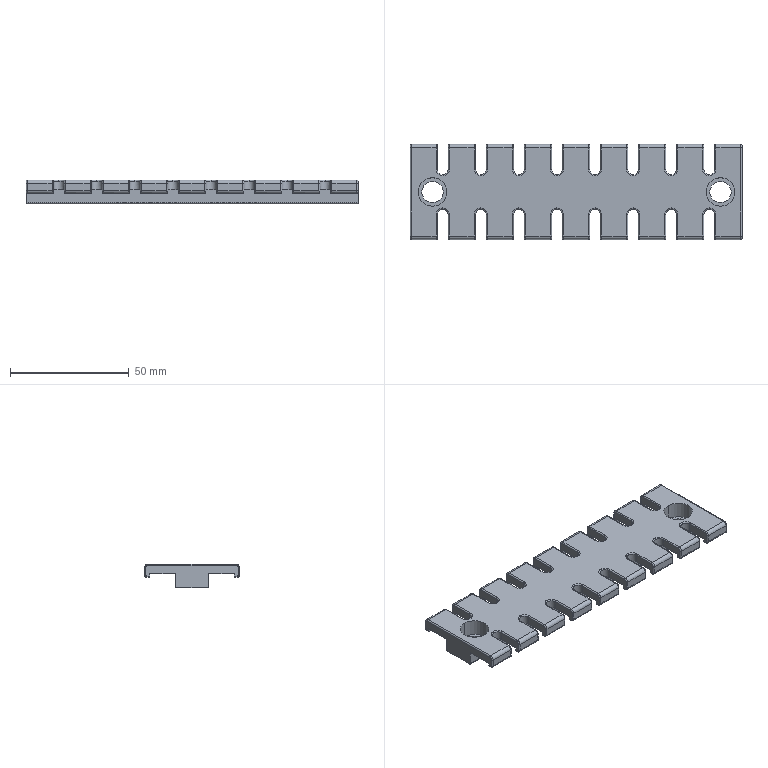Part | STEP file | ZL140 | 1 solid | 296 faces | box 139.5 x 40 x 10 mm | volume 29012 mm3 | cylinder 136 | plane 96 | torus 64 | commonest cylinder face diameters 1 x76 2 x18 3 x18 4.5 x16 9 x4 12 x4